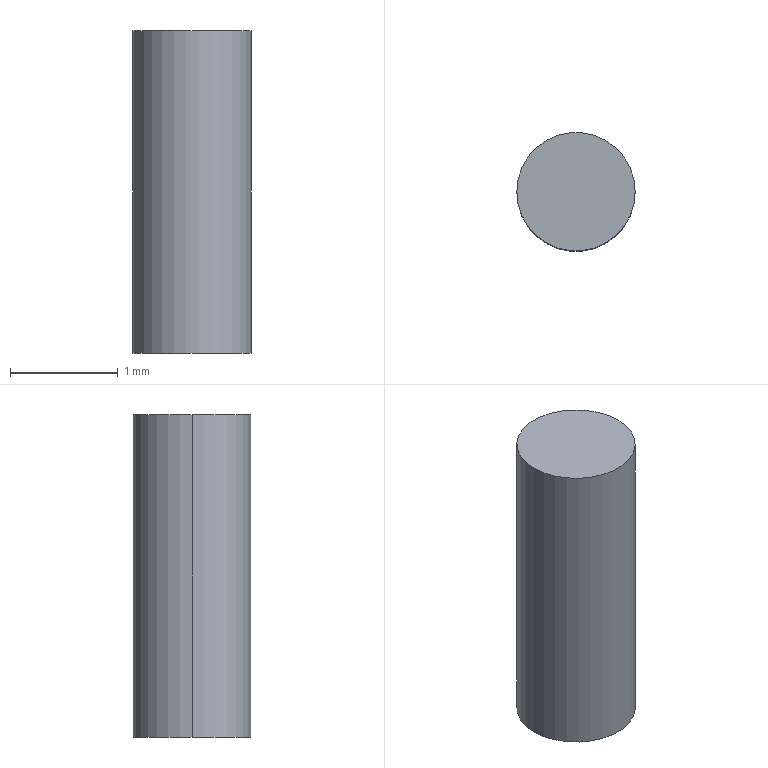Part | SolidWorks | features Extrusion 1 | 1 solid | 4 faces | box 1.1 x 1.1 x 3 mm | volume 2.851 mm3 | cylinder 2 | plane 2 | commonest cylinder face diameters 1.1 x2
STEP:
#1=CARTESIAN_POINT('',(0.55,0.,1.5));
#2=VERTEX_POINT('',#1);
#3=CARTESIAN_POINT('',(-0.55,0.,1.5));
#4=VERTEX_POINT('',#3);
#5=CARTESIAN_POINT('',(0.,0.,1.5));
#6=DIRECTION('',(0.,0.,1.));
#7=DIRECTION('',(1.,0.,0.));
#8=AXIS2_PLACEMENT_3D('',#5,#6,#7);
#9=CIRCLE('',#8,0.55);
#10=EDGE_CURVE('',#2,#4,#9,.T.);
#11=ORIENTED_EDGE('',*,*,#10,.F.);
#12=CARTESIAN_POINT('',(0.55,0.,-1.5));
#13=VERTEX_POINT('',#12);
#14=CARTESIAN_POINT('',(0.55,0.,1.5));
#15=DIRECTION('',(0.,0.,-1.));
#16=VECTOR('',#15,1000.);
#17=LINE('',#14,#16);
#18=EDGE_CURVE('',#2,#13,#17,.T.);
#19=ORIENTED_EDGE('',*,*,#18,.T.);
#20=CARTESIAN_POINT('',(-0.55,0.,-1.5));
#21=VERTEX_POINT('',#20);
#22=CARTESIAN_POINT('',(0.,0.,-1.5));
#23=DIRECTION('',(0.,0.,1.));
#24=DIRECTION('',(1.,0.,0.));
#25=AXIS2_PLACEMENT_3D('',#22,#23,#24);
#26=CIRCLE('',#25,0.55);
#27=EDGE_CURVE('',#13,#21,#26,.T.);
#28=ORIENTED_EDGE('',*,*,#27,.T.);
#29=CARTESIAN_POINT('',(-0.55,0.,1.5));
#30=DIRECTION('',(0.,0.,-1.));
#31=VECTOR('',#30,1000.);
#32=LINE('',#29,#31);
#33=EDGE_CURVE('',#4,#21,#32,.T.);
#34=ORIENTED_EDGE('',*,*,#33,.F.);
#35=EDGE_LOOP('',(#11,#19,#28,#34));
#36=FACE_OUTER_BOUND('',#35,.T.);
#37=CARTESIAN_POINT('',(0.,0.,1.5));
#38=DIRECTION('',(0.,0.,-1.));
#39=DIRECTION('',(-1.,0.,0.));
#40=AXIS2_PLACEMENT_3D('',#37,#38,#39);
#41=CYLINDRICAL_SURFACE('',#40,0.55);
#42=ADVANCED_FACE('',(#36),#41,.T.);
#43=ORIENTED_EDGE('',*,*,#18,.F.);
#44=CARTESIAN_POINT('',(0.,0.,1.5));
#45=DIRECTION('',(0.,0.,1.));
#46=DIRECTION('',(1.,0.,0.));
#47=AXIS2_PLACEMENT_3D('',#44,#45,#46);
#48=CIRCLE('',#47,0.55);
#49=EDGE_CURVE('',#4,#2,#48,.T.);
#50=ORIENTED_EDGE('',*,*,#49,.F.);
#51=ORIENTED_EDGE('',*,*,#33,.T.);
#52=CARTESIAN_POINT('',(0.,0.,-1.5));
#53=DIRECTION('',(0.,0.,1.));
#54=DIRECTION('',(1.,0.,0.));
#55=AXIS2_PLACEMENT_3D('',#52,#53,#54);
#56=CIRCLE('',#55,0.55);
#57=EDGE_CURVE('',#21,#13,#56,.T.);
#58=ORIENTED_EDGE('',*,*,#57,.T.);
#59=EDGE_LOOP('',(#43,#50,#51,#58));
#60=FACE_OUTER_BOUND('',#59,.T.);
#61=CARTESIAN_POINT('',(0.,0.,1.5));
#62=DIRECTION('',(0.,0.,-1.));
#63=DIRECTION('',(-1.,0.,0.));
#64=AXIS2_PLACEMENT_3D('',#61,#62,#63);
#65=CYLINDRICAL_SURFACE('',#64,0.55);
#66=ADVANCED_FACE('',(#60),#65,.T.);
#67=ORIENTED_EDGE('',*,*,#49,.T.);
#68=ORIENTED_EDGE('',*,*,#10,.T.);
#69=EDGE_LOOP('',(#67,#68));
#70=FACE_OUTER_BOUND('',#69,.T.);
#71=CARTESIAN_POINT('',(0.,0.,1.5));
#72=DIRECTION('',(0.,0.,1.));
#73=DIRECTION('',(1.,0.,0.));
#74=AXIS2_PLACEMENT_3D('',#71,#72,#73);
#75=PLANE('',#74);
#76=ADVANCED_FACE('',(#70),#75,.T.);
#77=ORIENTED_EDGE('',*,*,#57,.F.);
#78=ORIENTED_EDGE('',*,*,#27,.F.);
#79=EDGE_LOOP('',(#77,#78));
#80=FACE_OUTER_BOUND('',#79,.T.);
#81=CARTESIAN_POINT('',(0.,0.,-1.5));
#82=DIRECTION('',(0.,0.,1.));
#83=DIRECTION('',(1.,0.,0.));
#84=AXIS2_PLACEMENT_3D('',#81,#82,#83);
#85=PLANE('',#84);
#86=ADVANCED_FACE('',(#80),#85,.F.);
#87=CLOSED_SHELL('',(#42,#66,#76,#86));
#88=MANIFOLD_SOLID_BREP('',#87);
#89=CARTESIAN_POINT('',(0.,0.,0.));
#90=DIRECTION('',(0.,0.,1.));
#91=DIRECTION('',(1.,0.,0.));
#92=AXIS2_PLACEMENT_3D('',#89,#90,#91);
#93=(LENGTH_UNIT()NAMED_UNIT(*)SI_UNIT(.MILLI.,.METRE.));
#94=UNCERTAINTY_MEASURE_WITH_UNIT(LENGTH_MEASURE(0.00001),#93,'','');
#95=(NAMED_UNIT(*)PLANE_ANGLE_UNIT()SI_UNIT($,.RADIAN.));
#96=(NAMED_UNIT(*)SI_UNIT($,.STERADIAN.)SOLID_ANGLE_UNIT());
#97=(GEOMETRIC_REPRESENTATION_CONTEXT(3)GLOBAL_UNCERTAINTY_ASSIGNED_CONTEXT((#94))GLOBAL_UNIT_ASSIGNED_CONTEXT((#93,#95,#96))REPRESENTATION_CONTEXT('',''));
#98=ADVANCED_BREP_SHAPE_REPRESENTATION('',(#88,#92),#97);